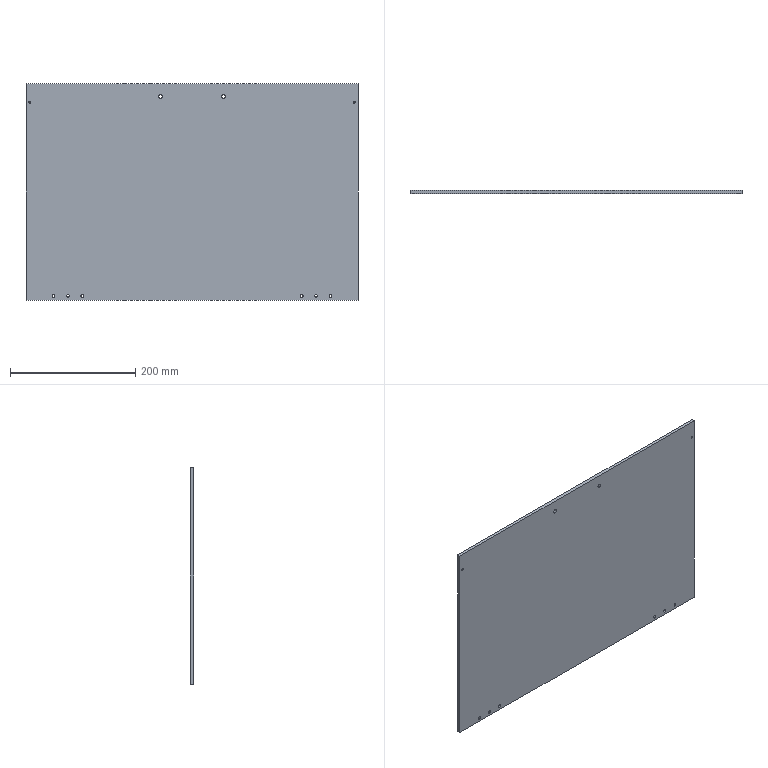Part | STEP file | OP10-034_shelf-door | 1 solid | 26 faces | box 530 x 5 x 345 mm | volume 913394 mm3 | cylinder 20 | plane 6 | commonest cylinder face diameters 4.5 x12 3.5 x4 6 x4